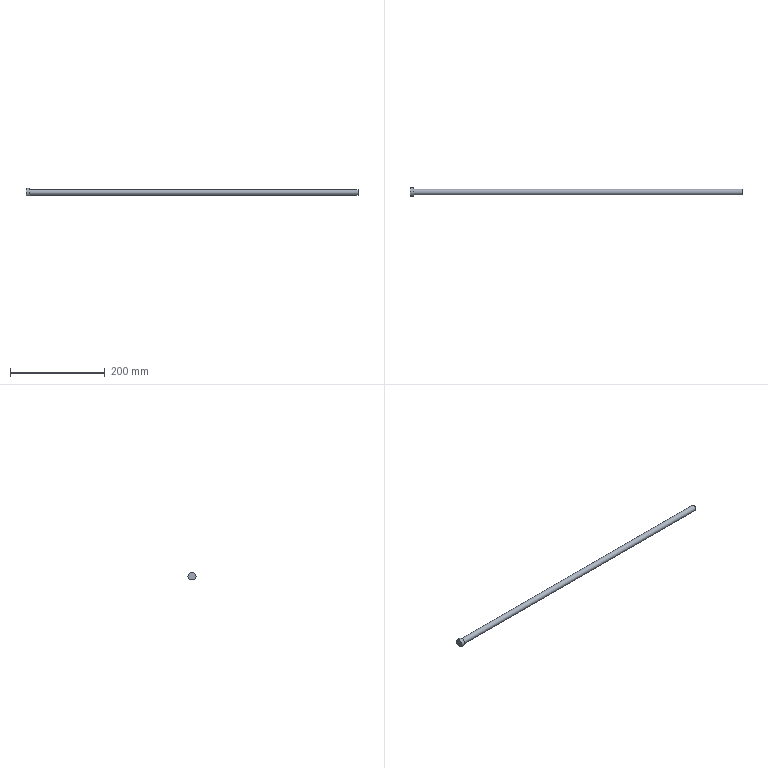Part | STEP file | solid 37 | 1 solid | 6 faces | box 700 x 17 x 15 mm | volume 79959 mm3 | plane 4 | cylinder 2 | commonest cylinder face diameters 12 x1 17 x1